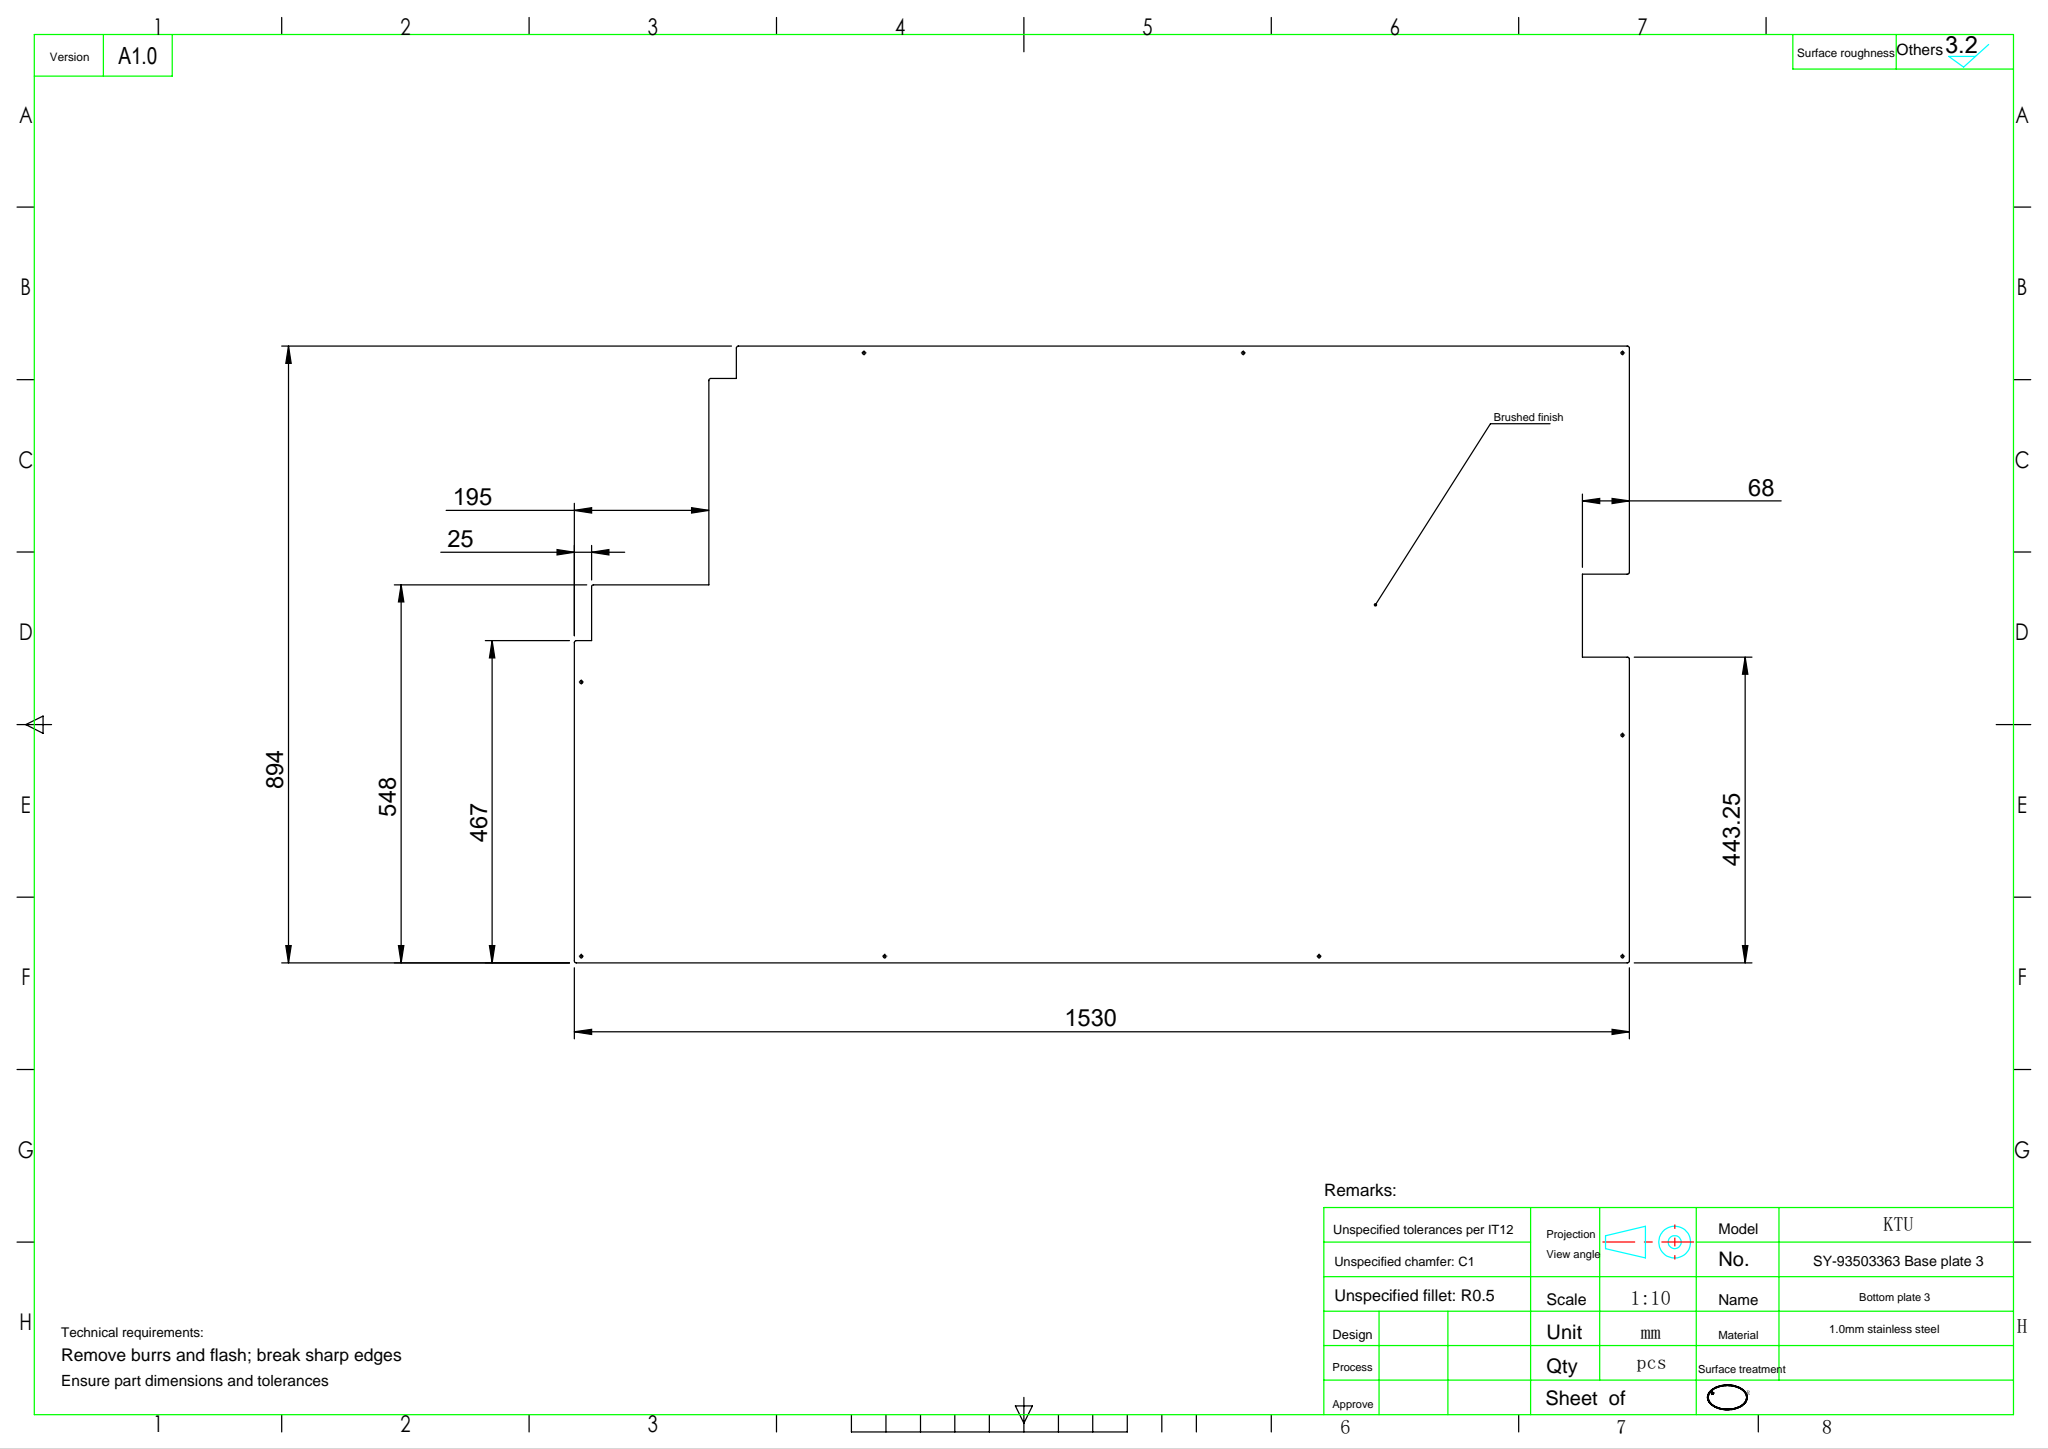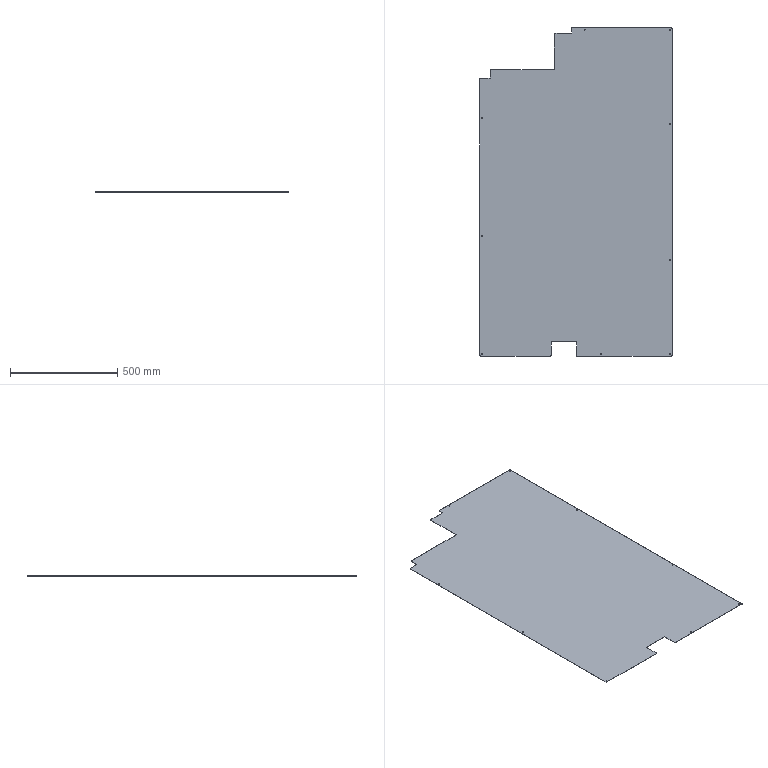Part | SolidWorks | features Cut 2, ICE 2, Fillet 1, FlatPattern 1, SMBaseFlange 1, SheetMetal 1 | 1 solid | 43 faces | box 894 x 1530 x 1 mm | volume 1288143 mm3 | cylinder 27 | plane 16 | commonest cylinder face diameters 4.2 x18 6 x9